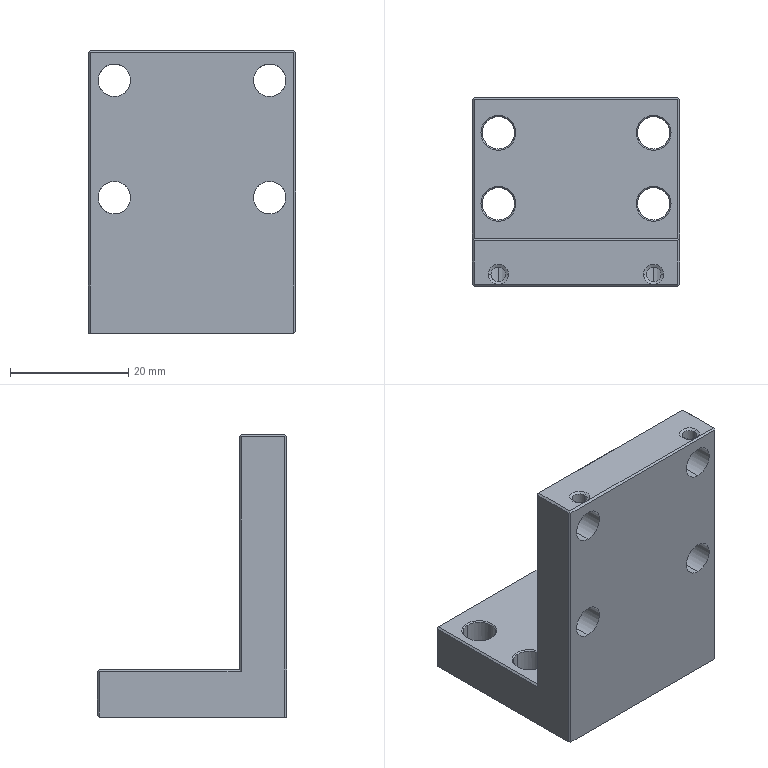Part | NX | 1 solid | 63 faces | box 35 x 32 x 47.7 mm | volume 18510 mm3 | plane 23 | cylinder 20 | cone 20 | commonest cylinder face diameters 5.5 x16 2.5 x4